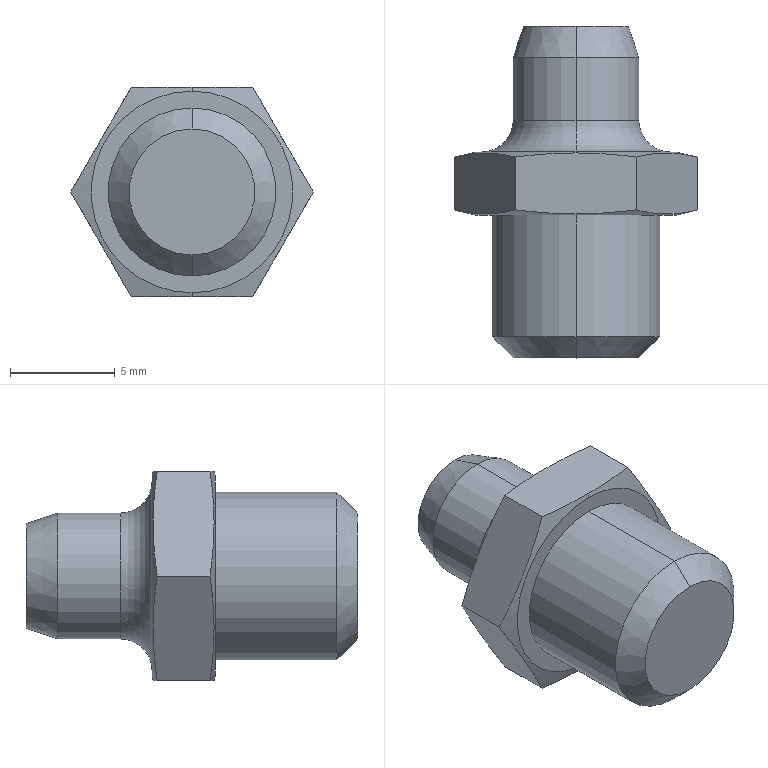Part | SolidWorks | features RevCut 2, Chamfer 1, Extrusion 1, ICE 1, Revolution 1 | 1 solid | 29 faces | box 11.547 x 15.8 x 10 mm | volume 760.457 mm3 | plane 11 | cone 10 | cylinder 4 | sphere 2 | torus 2 | commonest cylinder face diameters 6 x2 8 x2
STEP:
#1=CARTESIAN_POINT('',(0.,15.8,-0.8829));
#2=VERTEX_POINT('',#1);
#3=CARTESIAN_POINT('',(0.,15.8,0.8829));
#4=VERTEX_POINT('',#3);
#5=CARTESIAN_POINT('',(0.,15.8,0.));
#6=DIRECTION('',(0.,1.,0.));
#7=DIRECTION('',(0.,0.,1.));
#8=AXIS2_PLACEMENT_3D('',#5,#6,#7);
#9=CIRCLE('',#8,0.8829);
#10=EDGE_CURVE('',#2,#4,#9,.T.);
#11=ORIENTED_EDGE('',*,*,#10,.T.);
#12=CARTESIAN_POINT('',(0.,15.018,1.293));
#13=VERTEX_POINT('',#12);
#14=CARTESIAN_POINT('',(0.,15.018,1.293));
#15=DIRECTION('',(0.,-0.8855,0.4646));
#16=VECTOR('',#15,1000.);
#17=LINE('',#14,#16);
#18=EDGE_CURVE('',#4,#13,#17,.T.);
#19=ORIENTED_EDGE('',*,*,#18,.T.);
#20=CARTESIAN_POINT('',(0.,15.018,-1.293));
#21=VERTEX_POINT('',#20);
#22=CARTESIAN_POINT('',(0.,15.018,0.));
#23=DIRECTION('',(0.,1.,0.));
#24=DIRECTION('',(0.,0.,1.));
#25=AXIS2_PLACEMENT_3D('',#22,#23,#24);
#26=CIRCLE('',#25,1.293);
#27=EDGE_CURVE('',#21,#13,#26,.T.);
#28=ORIENTED_EDGE('',*,*,#27,.F.);
#29=CARTESIAN_POINT('',(0.,15.018,-1.293));
#30=DIRECTION('',(0.,-0.8855,-0.4646));
#31=VECTOR('',#30,1000.);
#32=LINE('',#29,#31);
#33=EDGE_CURVE('',#2,#21,#32,.T.);
#34=ORIENTED_EDGE('',*,*,#33,.F.);
#35=EDGE_LOOP('',(#11,#19,#28,#34));
#36=FACE_OUTER_BOUND('',#35,.T.);
#37=CARTESIAN_POINT('',(0.,15.018,0.));
#38=DIRECTION('',(0.,-1.,0.));
#39=DIRECTION('',(0.,0.,-1.));
#40=AXIS2_PLACEMENT_3D('',#37,#38,#39);
#41=CONICAL_SURFACE('',#40,1.293,0.4832);
#42=ADVANCED_FACE('',(#36),#41,.F.);
#43=CARTESIAN_POINT('',(0.,15.018,0.));
#44=DIRECTION('',(0.,1.,0.));
#45=DIRECTION('',(0.,0.,1.));
#46=AXIS2_PLACEMENT_3D('',#43,#44,#45);
#47=CIRCLE('',#46,1.293);
#48=EDGE_CURVE('',#13,#21,#47,.T.);
#49=ORIENTED_EDGE('',*,*,#48,.T.);
#50=CARTESIAN_POINT('',(0.,15.8,-0.02012));
#51=VERTEX_POINT('',#50);
#52=CARTESIAN_POINT('',(0.,14.34,0.));
#53=DIRECTION('',(1.,0.,0.));
#54=DIRECTION('',(0.,0.,-1.));
#55=AXIS2_PLACEMENT_3D('',#52,#53,#54);
#56=CIRCLE('',#55,1.46);
#57=EDGE_CURVE('',#21,#51,#56,.T.);
#58=ORIENTED_EDGE('',*,*,#57,.T.);
#59=CARTESIAN_POINT('',(0.,15.8,0.02012));
#60=VERTEX_POINT('',#59);
#61=CARTESIAN_POINT('',(0.,15.8,0.));
#62=DIRECTION('',(0.,1.,0.));
#63=DIRECTION('',(0.,0.,1.));
#64=AXIS2_PLACEMENT_3D('',#61,#62,#63);
#65=CIRCLE('',#64,0.02012);
#66=EDGE_CURVE('',#60,#51,#65,.T.);
#67=ORIENTED_EDGE('',*,*,#66,.F.);
#68=CARTESIAN_POINT('',(0.,14.34,0.));
#69=DIRECTION('',(-1.,0.,0.));
#70=DIRECTION('',(0.,0.,1.));
#71=AXIS2_PLACEMENT_3D('',#68,#69,#70);
#72=CIRCLE('',#71,1.46);
#73=EDGE_CURVE('',#13,#60,#72,.T.);
#74=ORIENTED_EDGE('',*,*,#73,.F.);
#75=EDGE_LOOP('',(#49,#58,#67,#74));
#76=FACE_OUTER_BOUND('',#75,.T.);
#77=CARTESIAN_POINT('',(0.,14.34,0.));
#78=DIRECTION('',(1.,0.,0.));
#79=DIRECTION('',(0.,0.,1.));
#80=AXIS2_PLACEMENT_3D('',#77,#78,#79);
#81=SPHERICAL_SURFACE('',#80,1.46);
#82=ADVANCED_FACE('',(#76),#81,.T.);
#83=CARTESIAN_POINT('',(0.,0.,-3.));
#84=VERTEX_POINT('',#83);
#85=CARTESIAN_POINT('',(0.,0.,3.));
#86=VERTEX_POINT('',#85);
#87=CARTESIAN_POINT('',(0.,0.,0.));
#88=DIRECTION('',(0.,-1.,0.));
#89=DIRECTION('',(0.,0.,1.));
#90=AXIS2_PLACEMENT_3D('',#87,#88,#89);
#91=CIRCLE('',#90,3.);
#92=EDGE_CURVE('',#84,#86,#91,.T.);
#93=ORIENTED_EDGE('',*,*,#92,.F.);
#94=CARTESIAN_POINT('',(0.,1.,-4.));
#95=VERTEX_POINT('',#94);
#96=CARTESIAN_POINT('',(0.,1.,-4.));
#97=DIRECTION('',(0.,0.7071,-0.7071));
#98=VECTOR('',#97,1000.);
#99=LINE('',#96,#98);
#100=EDGE_CURVE('',#84,#95,#99,.T.);
#101=ORIENTED_EDGE('',*,*,#100,.T.);
#102=CARTESIAN_POINT('',(0.,1.,4.));
#103=VERTEX_POINT('',#102);
#104=CARTESIAN_POINT('',(0.,1.,0.));
#105=DIRECTION('',(0.,1.,0.));
#106=DIRECTION('',(0.,0.,1.));
#107=AXIS2_PLACEMENT_3D('',#104,#105,#106);
#108=CIRCLE('',#107,4.);
#109=EDGE_CURVE('',#103,#95,#108,.T.);
#110=ORIENTED_EDGE('',*,*,#109,.F.);
#111=CARTESIAN_POINT('',(0.,1.,4.));
#112=DIRECTION('',(0.,0.7071,0.7071));
#113=VECTOR('',#112,1000.);
#114=LINE('',#111,#113);
#115=EDGE_CURVE('',#86,#103,#114,.T.);
#116=ORIENTED_EDGE('',*,*,#115,.F.);
#117=EDGE_LOOP('',(#93,#101,#110,#116));
#118=FACE_OUTER_BOUND('',#117,.T.);
#119=CARTESIAN_POINT('',(0.,1.,0.));
#120=DIRECTION('',(0.,1.,0.));
#121=DIRECTION('',(0.,0.,1.));
#122=AXIS2_PLACEMENT_3D('',#119,#120,#121);
#123=CONICAL_SURFACE('',#122,4.,0.7854);
#124=ADVANCED_FACE('',(#118),#123,.T.);
#125=CARTESIAN_POINT('',(0.,6.8,4.));
#126=VERTEX_POINT('',#125);
#127=CARTESIAN_POINT('',(0.,6.8,-4.));
#128=VERTEX_POINT('',#127);
#129=CARTESIAN_POINT('',(0.,6.8,0.));
#130=DIRECTION('',(0.,1.,0.));
#131=DIRECTION('',(0.,0.,1.));
#132=AXIS2_PLACEMENT_3D('',#129,#130,#131);
#133=CIRCLE('',#132,4.);
#134=EDGE_CURVE('',#126,#128,#133,.T.);
#135=ORIENTED_EDGE('',*,*,#134,.F.);
#136=CARTESIAN_POINT('',(0.,6.8,4.));
#137=DIRECTION('',(0.,-1.,0.));
#138=VECTOR('',#137,1000.);
#139=LINE('',#136,#138);
#140=EDGE_CURVE('',#126,#103,#139,.T.);
#141=ORIENTED_EDGE('',*,*,#140,.T.);
#142=ORIENTED_EDGE('',*,*,#109,.T.);
#143=CARTESIAN_POINT('',(0.,6.8,-4.));
#144=DIRECTION('',(0.,-1.,0.));
#145=VECTOR('',#144,1000.);
#146=LINE('',#143,#145);
#147=EDGE_CURVE('',#128,#95,#146,.T.);
#148=ORIENTED_EDGE('',*,*,#147,.F.);
#149=EDGE_LOOP('',(#135,#141,#142,#148));
#150=FACE_OUTER_BOUND('',#149,.T.);
#151=CARTESIAN_POINT('',(0.,6.8,0.));
#152=DIRECTION('',(0.,-1.,0.));
#153=DIRECTION('',(0.,0.,-1.));
#154=AXIS2_PLACEMENT_3D('',#151,#152,#153);
#155=CYLINDRICAL_SURFACE('',#154,4.);
#156=ADVANCED_FACE('',(#150),#155,.T.);
#157=CARTESIAN_POINT('',(0.,6.8,4.8));
#158=VERTEX_POINT('',#157);
#159=CARTESIAN_POINT('',(0.,6.8,-4.8));
#160=VERTEX_POINT('',#159);
#161=CARTESIAN_POINT('',(0.,6.8,0.));
#162=DIRECTION('',(0.,1.,0.));
#163=DIRECTION('',(0.,0.,1.));
#164=AXIS2_PLACEMENT_3D('',#161,#162,#163);
#165=CIRCLE('',#164,4.8);
#166=EDGE_CURVE('',#158,#160,#165,.T.);
#167=ORIENTED_EDGE('',*,*,#166,.T.);
#168=CARTESIAN_POINT('',(0.,6.85,-5.));
#169=VERTEX_POINT('',#168);
#170=CARTESIAN_POINT('',(0.,7.3,-6.8));
#171=DIRECTION('',(0.,0.2425,-0.9701));
#172=VECTOR('',#171,1000.);
#173=LINE('',#170,#172);
#174=EDGE_CURVE('',#160,#169,#173,.T.);
#175=ORIENTED_EDGE('',*,*,#174,.T.);
#176=CARTESIAN_POINT('',(2.887,7.043,-5.));
#177=VERTEX_POINT('',#176);
#178=CARTESIAN_POINT('',(0.,6.85,-5.));
#179=CARTESIAN_POINT('',(0.9585,6.85,-5.));
#180=CARTESIAN_POINT('',(1.929,6.924,-5.));
#181=CARTESIAN_POINT('',(2.887,7.043,-5.));
#182=B_SPLINE_CURVE_WITH_KNOTS('',3,(#178,#179,#180,#181),.UNSPECIFIED.,.F.,.F.,(4,4),(0.008769,0.01162),.UNSPECIFIED.);
#183=EDGE_CURVE('',#169,#177,#182,.T.);
#184=ORIENTED_EDGE('',*,*,#183,.T.);
#185=CARTESIAN_POINT('',(5.774,7.043,0.));
#186=VERTEX_POINT('',#185);
#187=CARTESIAN_POINT('',(2.887,7.043,-5.));
#188=CARTESIAN_POINT('',(3.368,6.923,-4.167));
#189=CARTESIAN_POINT('',(4.33,6.777,-2.5));
#190=CARTESIAN_POINT('',(5.292,6.923,-0.8333));
#191=CARTESIAN_POINT('',(5.774,7.043,0.));
#192=B_SPLINE_CURVE_WITH_KNOTS('',3,(#187,#188,#189,#190,#191),.UNSPECIFIED.,.F.,.F.,(4,1,4),(0.000000231,0.002887,0.005774),.UNSPECIFIED.);
#193=EDGE_CURVE('',#177,#186,#192,.T.);
#194=ORIENTED_EDGE('',*,*,#193,.T.);
#195=CARTESIAN_POINT('',(2.887,7.043,5.));
#196=VERTEX_POINT('',#195);
#197=CARTESIAN_POINT('',(5.774,7.043,0.));
#198=CARTESIAN_POINT('',(5.292,6.923,0.8333));
#199=CARTESIAN_POINT('',(4.33,6.777,2.5));
#200=CARTESIAN_POINT('',(3.368,6.923,4.167));
#201=CARTESIAN_POINT('',(2.887,7.043,5.));
#202=B_SPLINE_CURVE_WITH_KNOTS('',3,(#197,#198,#199,#200,#201),.UNSPECIFIED.,.F.,.F.,(4,1,4),(0.000000231,0.002887,0.005774),.UNSPECIFIED.);
#203=EDGE_CURVE('',#186,#196,#202,.T.);
#204=ORIENTED_EDGE('',*,*,#203,.T.);
#205=CARTESIAN_POINT('',(0.,6.85,5.));
#206=VERTEX_POINT('',#205);
#207=CARTESIAN_POINT('',(2.887,7.043,5.));
#208=CARTESIAN_POINT('',(1.931,6.924,5.));
#209=CARTESIAN_POINT('',(0.9699,6.85,5.));
#210=CARTESIAN_POINT('',(0.,6.85,5.));
#211=B_SPLINE_CURVE_WITH_KNOTS('',3,(#207,#208,#209,#210),.UNSPECIFIED.,.F.,.F.,(4,4),(0.00588,0.008769),.UNSPECIFIED.);
#212=EDGE_CURVE('',#196,#206,#211,.T.);
#213=ORIENTED_EDGE('',*,*,#212,.T.);
#214=CARTESIAN_POINT('',(0.,7.3,6.8));
#215=DIRECTION('',(0.,0.2425,0.9701));
#216=VECTOR('',#215,1000.);
#217=LINE('',#214,#216);
#218=EDGE_CURVE('',#158,#206,#217,.T.);
#219=ORIENTED_EDGE('',*,*,#218,.F.);
#220=EDGE_LOOP('',(#167,#175,#184,#194,#204,#213,#219));
#221=FACE_OUTER_BOUND('',#220,.T.);
#222=CARTESIAN_POINT('',(0.,7.3,0.));
#223=DIRECTION('',(0.,1.,0.));
#224=DIRECTION('',(0.,0.,1.));
#225=AXIS2_PLACEMENT_3D('',#222,#223,#224);
#226=CONICAL_SURFACE('',#225,6.8,1.326);
#227=ADVANCED_FACE('',(#221),#226,.T.);
#228=CARTESIAN_POINT('',(0.,9.8,4.8));
#229=VERTEX_POINT('',#228);
#230=CARTESIAN_POINT('',(0.,9.8,-4.8));
#231=VERTEX_POINT('',#230);
#232=CARTESIAN_POINT('',(0.,9.8,0.));
#233=DIRECTION('',(0.,1.,0.));
#234=DIRECTION('',(0.,0.,1.));
#235=AXIS2_PLACEMENT_3D('',#232,#233,#234);
#236=CIRCLE('',#235,4.8);
#237=EDGE_CURVE('',#229,#231,#236,.T.);
#238=ORIENTED_EDGE('',*,*,#237,.F.);
#239=CARTESIAN_POINT('',(0.,9.75,5.));
#240=VERTEX_POINT('',#239);
#241=CARTESIAN_POINT('',(0.,9.8,4.8));
#242=DIRECTION('',(0.,-0.2425,0.9701));
#243=VECTOR('',#242,1000.);
#244=LINE('',#241,#243);
#245=EDGE_CURVE('',#229,#240,#244,.T.);
#246=ORIENTED_EDGE('',*,*,#245,.T.);
#247=CARTESIAN_POINT('',(2.887,9.557,5.));
#248=VERTEX_POINT('',#247);
#249=CARTESIAN_POINT('',(0.,9.75,5.));
#250=CARTESIAN_POINT('',(0.9585,9.75,5.));
#251=CARTESIAN_POINT('',(1.929,9.676,5.));
#252=CARTESIAN_POINT('',(2.887,9.557,5.));
#253=B_SPLINE_CURVE_WITH_KNOTS('',3,(#249,#250,#251,#252),.UNSPECIFIED.,.F.,.F.,(4,4),(0.008769,0.01162),.UNSPECIFIED.);
#254=EDGE_CURVE('',#240,#248,#253,.T.);
#255=ORIENTED_EDGE('',*,*,#254,.T.);
#256=CARTESIAN_POINT('',(5.774,9.557,0.));
#257=VERTEX_POINT('',#256);
#258=CARTESIAN_POINT('',(2.887,9.557,5.));
#259=CARTESIAN_POINT('',(3.368,9.677,4.167));
#260=CARTESIAN_POINT('',(4.33,9.823,2.5));
#261=CARTESIAN_POINT('',(5.292,9.677,0.8333));
#262=CARTESIAN_POINT('',(5.774,9.557,0.));
#263=B_SPLINE_CURVE_WITH_KNOTS('',3,(#258,#259,#260,#261,#262),.UNSPECIFIED.,.F.,.F.,(4,1,4),(0.000000231,0.002887,0.005774),.UNSPECIFIED.);
#264=EDGE_CURVE('',#248,#257,#263,.T.);
#265=ORIENTED_EDGE('',*,*,#264,.T.);
#266=CARTESIAN_POINT('',(2.887,9.557,-5.));
#267=VERTEX_POINT('',#266);
#268=CARTESIAN_POINT('',(5.774,9.557,0.));
#269=CARTESIAN_POINT('',(5.292,9.677,-0.8333));
#270=CARTESIAN_POINT('',(4.33,9.823,-2.5));
#271=CARTESIAN_POINT('',(3.368,9.677,-4.167));
#272=CARTESIAN_POINT('',(2.887,9.557,-5.));
#273=B_SPLINE_CURVE_WITH_KNOTS('',3,(#268,#269,#270,#271,#272),.UNSPECIFIED.,.F.,.F.,(4,1,4),(0.000000231,0.002887,0.005774),.UNSPECIFIED.);
#274=EDGE_CURVE('',#257,#267,#273,.T.);
#275=ORIENTED_EDGE('',*,*,#274,.T.);
#276=CARTESIAN_POINT('',(0.,9.75,-5.));
#277=VERTEX_POINT('',#276);
#278=CARTESIAN_POINT('',(2.887,9.557,-5.));
#279=CARTESIAN_POINT('',(1.931,9.676,-5.));
#280=CARTESIAN_POINT('',(0.9699,9.75,-5.));
#281=CARTESIAN_POINT('',(0.,9.75,-5.));
#282=B_SPLINE_CURVE_WITH_KNOTS('',3,(#278,#279,#280,#281),.UNSPECIFIED.,.F.,.F.,(4,4),(0.00588,0.008769),.UNSPECIFIED.);
#283=EDGE_CURVE('',#267,#277,#282,.T.);
#284=ORIENTED_EDGE('',*,*,#283,.T.);
#285=CARTESIAN_POINT('',(0.,9.8,-4.8));
#286=DIRECTION('',(0.,-0.2425,-0.9701));
#287=VECTOR('',#286,1000.);
#288=LINE('',#285,#287);
#289=EDGE_CURVE('',#231,#277,#288,.T.);
#290=ORIENTED_EDGE('',*,*,#289,.F.);
#291=EDGE_LOOP('',(#238,#246,#255,#265,#275,#284,#290));
#292=FACE_OUTER_BOUND('',#291,.T.);
#293=CARTESIAN_POINT('',(0.,9.8,0.));
#294=DIRECTION('',(0.,-1.,0.));
#295=DIRECTION('',(0.,0.,-1.));
#296=AXIS2_PLACEMENT_3D('',#293,#294,#295);
#297=CONICAL_SURFACE('',#296,4.8,1.326);
#298=ADVANCED_FACE('',(#292),#297,.T.);
#299=CARTESIAN_POINT('',(0.,15.8,-2.5));
#300=VERTEX_POINT('',#299);
#301=CARTESIAN_POINT('',(0.,15.8,2.5));
#302=VERTEX_POINT('',#301);
#303=CARTESIAN_POINT('',(0.,15.8,0.));
#304=DIRECTION('',(0.,-1.,0.));
#305=DIRECTION('',(0.,0.,-1.));
#306=AXIS2_PLACEMENT_3D('',#303,#304,#305);
#307=CIRCLE('',#306,2.5);
#308=EDGE_CURVE('',#300,#302,#307,.T.);
#309=ORIENTED_EDGE('',*,*,#308,.T.);
#310=CARTESIAN_POINT('',(0.,14.3,3.));
#311=VERTEX_POINT('',#310);
#312=CARTESIAN_POINT('',(0.,15.8,2.5));
#313=DIRECTION('',(0.,-0.9487,0.3162));
#314=VECTOR('',#313,1000.);
#315=LINE('',#312,#314);
#316=EDGE_CURVE('',#302,#311,#315,.T.);
#317=ORIENTED_EDGE('',*,*,#316,.T.);
#318=CARTESIAN_POINT('',(0.,14.3,-3.));
#319=VERTEX_POINT('',#318);
#320=CARTESIAN_POINT('',(0.,14.3,0.));
#321=DIRECTION('',(0.,-1.,0.));
#322=DIRECTION('',(0.,0.,-1.));
#323=AXIS2_PLACEMENT_3D('',#320,#321,#322);
#324=CIRCLE('',#323,3.);
#325=EDGE_CURVE('',#319,#311,#324,.T.);
#326=ORIENTED_EDGE('',*,*,#325,.F.);
#327=CARTESIAN_POINT('',(0.,15.8,-2.5));
#328=DIRECTION('',(0.,-0.9487,-0.3162));
#329=VECTOR('',#328,1000.);
#330=LINE('',#327,#329);
#331=EDGE_CURVE('',#300,#319,#330,.T.);
#332=ORIENTED_EDGE('',*,*,#331,.F.);
#333=EDGE_LOOP('',(#309,#317,#326,#332));
#334=FACE_OUTER_BOUND('',#333,.T.);
#335=CARTESIAN_POINT('',(0.,15.8,0.));
#336=DIRECTION('',(0.,-1.,0.));
#337=DIRECTION('',(0.,0.,-1.));
#338=AXIS2_PLACEMENT_3D('',#335,#336,#337);
#339=CONICAL_SURFACE('',#338,2.5,0.3218);
#340=ADVANCED_FACE('',(#334),#339,.T.);
#341=ORIENTED_EDGE('',*,*,#325,.T.);
#342=CARTESIAN_POINT('',(0.,11.3,3.));
#343=VERTEX_POINT('',#342);
#344=CARTESIAN_POINT('',(0.,-1.88,3.));
#345=DIRECTION('',(0.,-1.,0.));
#346=VECTOR('',#345,1000.);
#347=LINE('',#344,#346);
#348=EDGE_CURVE('',#311,#343,#347,.T.);
#349=ORIENTED_EDGE('',*,*,#348,.T.);
#350=CARTESIAN_POINT('',(0.,11.3,-3.));
#351=VERTEX_POINT('',#350);
#352=CARTESIAN_POINT('',(0.,11.3,0.));
#353=DIRECTION('',(0.,-1.,0.));
#354=DIRECTION('',(0.,0.,-1.));
#355=AXIS2_PLACEMENT_3D('',#352,#353,#354);
#356=CIRCLE('',#355,3.);
#357=EDGE_CURVE('',#351,#343,#356,.T.);
#358=ORIENTED_EDGE('',*,*,#357,.F.);
#359=CARTESIAN_POINT('',(0.,-1.88,-3.));
#360=DIRECTION('',(0.,-1.,0.));
#361=VECTOR('',#360,1000.);
#362=LINE('',#359,#361);
#363=EDGE_CURVE('',#319,#351,#362,.T.);
#364=ORIENTED_EDGE('',*,*,#363,.F.);
#365=EDGE_LOOP('',(#341,#349,#358,#364));
#366=FACE_OUTER_BOUND('',#365,.T.);
#367=CARTESIAN_POINT('',(0.,-1.88,0.));
#368=DIRECTION('',(0.,-1.,0.));
#369=DIRECTION('',(0.,0.,-1.));
#370=AXIS2_PLACEMENT_3D('',#367,#368,#369);
#371=CYLINDRICAL_SURFACE('',#370,3.);
#372=ADVANCED_FACE('',(#366),#371,.T.);
#373=CARTESIAN_POINT('',(0.,9.8,4.5));
#374=VERTEX_POINT('',#373);
#375=CARTESIAN_POINT('',(0.,9.8,-4.5));
#376=VERTEX_POINT('',#375);
#377=CARTESIAN_POINT('',(0.,9.8,0.));
#378=DIRECTION('',(0.,-1.,0.));
#379=DIRECTION('',(0.,0.,-1.));
#380=AXIS2_PLACEMENT_3D('',#377,#378,#379);
#381=CIRCLE('',#380,4.5);
#382=EDGE_CURVE('',#374,#376,#381,.T.);
#383=ORIENTED_EDGE('',*,*,#382,.F.);
#384=CARTESIAN_POINT('',(0.,11.3,4.5));
#385=DIRECTION('',(1.,0.,0.));
#386=DIRECTION('',(0.,0.,-1.));
#387=AXIS2_PLACEMENT_3D('',#384,#385,#386);
#388=CIRCLE('',#387,1.5);
#389=EDGE_CURVE('',#374,#343,#388,.T.);
#390=ORIENTED_EDGE('',*,*,#389,.T.);
#391=CARTESIAN_POINT('',(0.,11.3,0.));
#392=DIRECTION('',(0.,-1.,0.));
#393=DIRECTION('',(0.,0.,-1.));
#394=AXIS2_PLACEMENT_3D('',#391,#392,#393);
#395=CIRCLE('',#394,3.);
#396=EDGE_CURVE('',#343,#351,#395,.T.);
#397=ORIENTED_EDGE('',*,*,#396,.T.);
#398=CARTESIAN_POINT('',(0.,11.3,-4.5));
#399=DIRECTION('',(-1.,0.,0.));
#400=DIRECTION('',(0.,0.,1.));
#401=AXIS2_PLACEMENT_3D('',#398,#399,#400);
#402=CIRCLE('',#401,1.5);
#403=EDGE_CURVE('',#376,#351,#402,.T.);
#404=ORIENTED_EDGE('',*,*,#403,.F.);
#405=EDGE_LOOP('',(#383,#390,#397,#404));
#406=FACE_OUTER_BOUND('',#405,.T.);
#407=CARTESIAN_POINT('',(0.,11.3,0.));
#408=DIRECTION('',(0.,-1.,0.));
#409=DIRECTION('',(0.,0.,-1.));
#410=AXIS2_PLACEMENT_3D('',#407,#408,#409);
#411=TOROIDAL_SURFACE('',#410,4.5,1.5);
#412=ADVANCED_FACE('',(#406),#411,.F.);
#413=CARTESIAN_POINT('',(0.,9.8,0.));
#414=DIRECTION('',(0.,-1.,0.));
#415=DIRECTION('',(0.,0.,-1.));
#416=AXIS2_PLACEMENT_3D('',#413,#414,#415);
#417=CIRCLE('',#416,4.5);
#418=EDGE_CURVE('',#376,#374,#417,.T.);
#419=ORIENTED_EDGE('',*,*,#418,.T.);
#420=ORIENTED_EDGE('',*,*,#382,.T.);
#421=EDGE_LOOP('',(#419,#420));
#422=FACE_BOUND('',#421,.T.);
#423=CARTESIAN_POINT('',(0.,9.8,0.));
#424=DIRECTION('',(0.,1.,0.));
#425=DIRECTION('',(0.,0.,1.));
#426=AXIS2_PLACEMENT_3D('',#423,#424,#425);
#427=CIRCLE('',#426,4.8);
#428=EDGE_CURVE('',#231,#229,#427,.T.);
#429=ORIENTED_EDGE('',*,*,#428,.T.);
#430=ORIENTED_EDGE('',*,*,#237,.T.);
#431=EDGE_LOOP('',(#429,#430));
#432=FACE_OUTER_BOUND('',#431,.T.);
#433=CARTESIAN_POINT('',(0.,9.8,0.));
#434=DIRECTION('',(0.,1.,0.));
#435=DIRECTION('',(0.,0.,1.));
#436=AXIS2_PLACEMENT_3D('',#433,#434,#435);
#437=PLANE('',#436);
#438=ADVANCED_FACE('',(#422,#432),#437,.T.);
#439=ORIENTED_EDGE('',*,*,#389,.F.);
#440=ORIENTED_EDGE('',*,*,#418,.F.);
#441=ORIENTED_EDGE('',*,*,#403,.T.);
#442=ORIENTED_EDGE('',*,*,#357,.T.);
#443=EDGE_LOOP('',(#439,#440,#441,#442));
#444=FACE_OUTER_BOUND('',#443,.T.);
#445=CARTESIAN_POINT('',(0.,11.3,0.));
#446=DIRECTION('',(0.,-1.,0.));
#447=DIRECTION('',(0.,0.,-1.));
#448=AXIS2_PLACEMENT_3D('',#445,#446,#447);
#449=TOROIDAL_SURFACE('',#448,4.5,1.5);
#450=ADVANCED_FACE('',(#444),#449,.F.);
#451=ORIENTED_EDGE('',*,*,#348,.F.);
#452=CARTESIAN_POINT('',(0.,14.3,0.));
#453=DIRECTION('',(0.,-1.,0.));
#454=DIRECTION('',(0.,0.,-1.));
#455=AXIS2_PLACEMENT_3D('',#452,#453,#454);
#456=CIRCLE('',#455,3.);
#457=EDGE_CURVE('',#311,#319,#456,.T.);
#458=ORIENTED_EDGE('',*,*,#457,.T.);
#459=ORIENTED_EDGE('',*,*,#363,.T.);
#460=ORIENTED_EDGE('',*,*,#396,.F.);
#461=EDGE_LOOP('',(#451,#458,#459,#460));
#462=FACE_OUTER_BOUND('',#461,.T.);
#463=CARTESIAN_POINT('',(0.,-1.88,0.));
#464=DIRECTION('',(0.,-1.,0.));
#465=DIRECTION('',(0.,0.,-1.));
#466=AXIS2_PLACEMENT_3D('',#463,#464,#465);
#467=CYLINDRICAL_SURFACE('',#466,3.);
#468=ADVANCED_FACE('',(#462),#467,.T.);
#469=ORIENTED_EDGE('',*,*,#316,.F.);
#470=CARTESIAN_POINT('',(0.,15.8,0.));
#471=DIRECTION('',(0.,-1.,0.));
#472=DIRECTION('',(0.,0.,-1.));
#473=AXIS2_PLACEMENT_3D('',#470,#471,#472);
#474=CIRCLE('',#473,2.5);
#475=EDGE_CURVE('',#302,#300,#474,.T.);
#476=ORIENTED_EDGE('',*,*,#475,.T.);
#477=ORIENTED_EDGE('',*,*,#331,.T.);
#478=ORIENTED_EDGE('',*,*,#457,.F.);
#479=EDGE_LOOP('',(#469,#476,#477,#478));
#480=FACE_OUTER_BOUND('',#479,.T.);
#481=CARTESIAN_POINT('',(0.,15.8,0.));
#482=DIRECTION('',(0.,-1.,0.));
#483=DIRECTION('',(0.,0.,-1.));
#484=AXIS2_PLACEMENT_3D('',#481,#482,#483);
#485=CONICAL_SURFACE('',#484,2.5,0.3218);
#486=ADVANCED_FACE('',(#480),#485,.T.);
#487=ORIENTED_EDGE('',*,*,#10,.F.);
#488=CARTESIAN_POINT('',(0.,15.8,0.));
#489=DIRECTION('',(0.,1.,0.));
#490=DIRECTION('',(0.,0.,1.));
#491=AXIS2_PLACEMENT_3D('',#488,#489,#490);
#492=CIRCLE('',#491,0.8829);
#493=EDGE_CURVE('',#4,#2,#492,.T.);
#494=ORIENTED_EDGE('',*,*,#493,.F.);
#495=EDGE_LOOP('',(#487,#494));
#496=FACE_BOUND('',#495,.T.);
#497=ORIENTED_EDGE('',*,*,#308,.F.);
#498=ORIENTED_EDGE('',*,*,#475,.F.);
#499=EDGE_LOOP('',(#497,#498));
#500=FACE_OUTER_BOUND('',#499,.T.);
#501=CARTESIAN_POINT('',(0.,15.8,0.));
#502=DIRECTION('',(0.,-1.,0.));
#503=DIRECTION('',(0.,0.,-1.));
#504=AXIS2_PLACEMENT_3D('',#501,#502,#503);
#505=PLANE('',#504);
#506=ADVANCED_FACE('',(#496,#500),#505,.F.);
#507=ORIENTED_EDGE('',*,*,#245,.F.);
#508=ORIENTED_EDGE('',*,*,#428,.F.);
#509=ORIENTED_EDGE('',*,*,#289,.T.);
#510=CARTESIAN_POINT('',(-2.887,9.557,-5.));
#511=VERTEX_POINT('',#510);
#512=CARTESIAN_POINT('',(0.,9.75,-5.));
#513=CARTESIAN_POINT('',(-0.9585,9.75,-5.));
#514=CARTESIAN_POINT('',(-1.929,9.676,-5.));
#515=CARTESIAN_POINT('',(-2.887,9.557,-5.));
#516=B_SPLINE_CURVE_WITH_KNOTS('',3,(#512,#513,#514,#515),.UNSPECIFIED.,.F.,.F.,(4,4),(0.008769,0.01162),.UNSPECIFIED.);
#517=EDGE_CURVE('',#277,#511,#516,.T.);
#518=ORIENTED_EDGE('',*,*,#517,.T.);
#519=CARTESIAN_POINT('',(-5.774,9.557,0.));
#520=VERTEX_POINT('',#519);
#521=CARTESIAN_POINT('',(-2.887,9.557,-5.));
#522=CARTESIAN_POINT('',(-3.368,9.677,-4.167));
#523=CARTESIAN_POINT('',(-4.33,9.823,-2.5));
#524=CARTESIAN_POINT('',(-5.292,9.677,-0.8333));
#525=CARTESIAN_POINT('',(-5.774,9.557,0.));
#526=B_SPLINE_CURVE_WITH_KNOTS('',3,(#521,#522,#523,#524,#525),.UNSPECIFIED.,.F.,.F.,(4,1,4),(0.000000231,0.002887,0.005774),.UNSPECIFIED.);
#527=EDGE_CURVE('',#511,#520,#526,.T.);
#528=ORIENTED_EDGE('',*,*,#527,.T.);
#529=CARTESIAN_POINT('',(-2.887,9.557,5.));
#530=VERTEX_POINT('',#529);
#531=CARTESIAN_POINT('',(-5.774,9.557,0.));
#532=CARTESIAN_POINT('',(-5.292,9.677,0.8333));
#533=CARTESIAN_POINT('',(-4.33,9.823,2.5));
#534=CARTESIAN_POINT('',(-3.368,9.677,4.167));
#535=CARTESIAN_POINT('',(-2.887,9.557,5.));
#536=B_SPLINE_CURVE_WITH_KNOTS('',3,(#531,#532,#533,#534,#535),.UNSPECIFIED.,.F.,.F.,(4,1,4),(0.000000231,0.002887,0.005774),.UNSPECIFIED.);
#537=EDGE_CURVE('',#520,#530,#536,.T.);
#538=ORIENTED_EDGE('',*,*,#537,.T.);
#539=CARTESIAN_POINT('',(-2.887,9.557,5.));
#540=CARTESIAN_POINT('',(-1.931,9.676,5.));
#541=CARTESIAN_POINT('',(-0.9699,9.75,5.));
#542=CARTESIAN_POINT('',(0.,9.75,5.));
#543=B_SPLINE_CURVE_WITH_KNOTS('',3,(#539,#540,#541,#542),.UNSPECIFIED.,.F.,.F.,(4,4),(0.00588,0.008769),.UNSPECIFIED.);
#544=EDGE_CURVE('',#530,#240,#543,.T.);
#545=ORIENTED_EDGE('',*,*,#544,.T.);
#546=EDGE_LOOP('',(#507,#508,#509,#518,#528,#538,#545));
#547=FACE_OUTER_BOUND('',#546,.T.);
#548=CARTESIAN_POINT('',(0.,9.8,0.));
#549=DIRECTION('',(0.,-1.,0.));
#550=DIRECTION('',(0.,0.,-1.));
#551=AXIS2_PLACEMENT_3D('',#548,#549,#550);
#552=CONICAL_SURFACE('',#551,4.8,1.326);
#553=ADVANCED_FACE('',(#547),#552,.T.);
#554=ORIENTED_EDGE('',*,*,#537,.F.);
#555=CARTESIAN_POINT('',(-5.774,7.043,0.));
#556=VERTEX_POINT('',#555);
#557=CARTESIAN_POINT('',(-5.774,9.8,0.));
#558=DIRECTION('',(0.,-1.,0.));
#559=VECTOR('',#558,1000.);
#560=LINE('',#557,#559);
#561=EDGE_CURVE('',#520,#556,#560,.T.);
#562=ORIENTED_EDGE('',*,*,#561,.T.);
#563=CARTESIAN_POINT('',(-2.887,7.043,5.));
#564=VERTEX_POINT('',#563);
#565=CARTESIAN_POINT('',(-2.887,7.043,5.));
#566=CARTESIAN_POINT('',(-3.368,6.923,4.167));
#567=CARTESIAN_POINT('',(-4.33,6.777,2.5));
#568=CARTESIAN_POINT('',(-5.292,6.923,0.8333));
#569=CARTESIAN_POINT('',(-5.774,7.043,0.));
#570=B_SPLINE_CURVE_WITH_KNOTS('',3,(#565,#566,#567,#568,#569),.UNSPECIFIED.,.F.,.F.,(4,1,4),(0.000000231,0.002887,0.005774),.UNSPECIFIED.);
#571=EDGE_CURVE('',#564,#556,#570,.T.);
#572=ORIENTED_EDGE('',*,*,#571,.F.);
#573=CARTESIAN_POINT('',(-2.887,9.8,5.));
#574=DIRECTION('',(0.,-1.,0.));
#575=VECTOR('',#574,1000.);
#576=LINE('',#573,#575);
#577=EDGE_CURVE('',#530,#564,#576,.T.);
#578=ORIENTED_EDGE('',*,*,#577,.F.);
#579=EDGE_LOOP('',(#554,#562,#572,#578));
#580=FACE_OUTER_BOUND('',#579,.T.);
#581=CARTESIAN_POINT('',(-5.774,9.8,0.));
#582=DIRECTION('',(0.866,0.,-0.5));
#583=DIRECTION('',(-0.5,0.,-0.866));
#584=AXIS2_PLACEMENT_3D('',#581,#582,#583);
#585=PLANE('',#584);
#586=ADVANCED_FACE('',(#580),#585,.F.);
#587=ORIENTED_EDGE('',*,*,#527,.F.);
#588=CARTESIAN_POINT('',(-2.887,7.043,-5.));
#589=VERTEX_POINT('',#588);
#590=CARTESIAN_POINT('',(-2.887,9.8,-5.));
#591=DIRECTION('',(0.,-1.,0.));
#592=VECTOR('',#591,1000.);
#593=LINE('',#590,#592);
#594=EDGE_CURVE('',#511,#589,#593,.T.);
#595=ORIENTED_EDGE('',*,*,#594,.T.);
#596=CARTESIAN_POINT('',(-5.774,7.043,0.));
#597=CARTESIAN_POINT('',(-5.292,6.923,-0.8333));
#598=CARTESIAN_POINT('',(-4.33,6.777,-2.5));
#599=CARTESIAN_POINT('',(-3.368,6.923,-4.167));
#600=CARTESIAN_POINT('',(-2.887,7.043,-5.));
#601=B_SPLINE_CURVE_WITH_KNOTS('',3,(#596,#597,#598,#599,#600),.UNSPECIFIED.,.F.,.F.,(4,1,4),(0.000000231,0.002887,0.005774),.UNSPECIFIED.);
#602=EDGE_CURVE('',#556,#589,#601,.T.);
#603=ORIENTED_EDGE('',*,*,#602,.F.);
#604=ORIENTED_EDGE('',*,*,#561,.F.);
#605=EDGE_LOOP('',(#587,#595,#603,#604));
#606=FACE_OUTER_BOUND('',#605,.T.);
#607=CARTESIAN_POINT('',(-2.887,9.8,-5.));
#608=DIRECTION('',(0.866,0.,0.5));
#609=DIRECTION('',(0.5,0.,-0.866));
#610=AXIS2_PLACEMENT_3D('',#607,#608,#609);
#611=PLANE('',#610);
#612=ADVANCED_FACE('',(#606),#611,.F.);
#613=ORIENTED_EDGE('',*,*,#283,.F.);
#614=CARTESIAN_POINT('',(2.887,9.8,-5.));
#615=DIRECTION('',(0.,-1.,0.));
#616=VECTOR('',#615,1000.);
#617=LINE('',#614,#616);
#618=EDGE_CURVE('',#267,#177,#617,.T.);
#619=ORIENTED_EDGE('',*,*,#618,.T.);
#620=ORIENTED_EDGE('',*,*,#183,.F.);
#621=CARTESIAN_POINT('',(-2.887,7.043,-5.));
#622=CARTESIAN_POINT('',(-1.931,6.924,-5.));
#623=CARTESIAN_POINT('',(-0.9699,6.85,-5.));
#624=CARTESIAN_POINT('',(0.,6.85,-5.));
#625=B_SPLINE_CURVE_WITH_KNOTS('',3,(#621,#622,#623,#624),.UNSPECIFIED.,.F.,.F.,(4,4),(0.00588,0.008769),.UNSPECIFIED.);
#626=EDGE_CURVE('',#589,#169,#625,.T.);
#627=ORIENTED_EDGE('',*,*,#626,.F.);
#628=ORIENTED_EDGE('',*,*,#594,.F.);
#629=ORIENTED_EDGE('',*,*,#517,.F.);
#630=EDGE_LOOP('',(#613,#619,#620,#627,#628,#629));
#631=FACE_OUTER_BOUND('',#630,.T.);
#632=CARTESIAN_POINT('',(2.887,9.8,-5.));
#633=DIRECTION('',(0.,0.,1.));
#634=DIRECTION('',(1.,0.,0.));
#635=AXIS2_PLACEMENT_3D('',#632,#633,#634);
#636=PLANE('',#635);
#637=ADVANCED_FACE('',(#631),#636,.F.);
#638=ORIENTED_EDGE('',*,*,#274,.F.);
#639=CARTESIAN_POINT('',(5.774,9.8,0.));
#640=DIRECTION('',(0.,-1.,0.));
#641=VECTOR('',#640,1000.);
#642=LINE('',#639,#641);
#643=EDGE_CURVE('',#257,#186,#642,.T.);
#644=ORIENTED_EDGE('',*,*,#643,.T.);
#645=ORIENTED_EDGE('',*,*,#193,.F.);
#646=ORIENTED_EDGE('',*,*,#618,.F.);
#647=EDGE_LOOP('',(#638,#644,#645,#646));
#648=FACE_OUTER_BOUND('',#647,.T.);
#649=CARTESIAN_POINT('',(5.774,9.8,0.));
#650=DIRECTION('',(-0.866,0.,0.5));
#651=DIRECTION('',(0.5,0.,0.866));
#652=AXIS2_PLACEMENT_3D('',#649,#650,#651);
#653=PLANE('',#652);
#654=ADVANCED_FACE('',(#648),#653,.F.);
#655=ORIENTED_EDGE('',*,*,#264,.F.);
#656=CARTESIAN_POINT('',(2.887,9.8,5.));
#657=DIRECTION('',(0.,-1.,0.));
#658=VECTOR('',#657,1000.);
#659=LINE('',#656,#658);
#660=EDGE_CURVE('',#248,#196,#659,.T.);
#661=ORIENTED_EDGE('',*,*,#660,.T.);
#662=ORIENTED_EDGE('',*,*,#203,.F.);
#663=ORIENTED_EDGE('',*,*,#643,.F.);
#664=EDGE_LOOP('',(#655,#661,#662,#663));
#665=FACE_OUTER_BOUND('',#664,.T.);
#666=CARTESIAN_POINT('',(2.887,9.8,5.));
#667=DIRECTION('',(-0.866,0.,-0.5));
#668=DIRECTION('',(-0.5,0.,0.866));
#669=AXIS2_PLACEMENT_3D('',#666,#667,#668);
#670=PLANE('',#669);
#671=ADVANCED_FACE('',(#665),#670,.F.);
#672=ORIENTED_EDGE('',*,*,#544,.F.);
#673=ORIENTED_EDGE('',*,*,#577,.T.);
#674=CARTESIAN_POINT('',(0.,6.85,5.));
#675=CARTESIAN_POINT('',(-0.9585,6.85,5.));
#676=CARTESIAN_POINT('',(-1.929,6.924,5.));
#677=CARTESIAN_POINT('',(-2.887,7.043,5.));
#678=B_SPLINE_CURVE_WITH_KNOTS('',3,(#674,#675,#676,#677),.UNSPECIFIED.,.F.,.F.,(4,4),(0.008769,0.01162),.UNSPECIFIED.);
#679=EDGE_CURVE('',#206,#564,#678,.T.);
#680=ORIENTED_EDGE('',*,*,#679,.F.);
#681=ORIENTED_EDGE('',*,*,#212,.F.);
#682=ORIENTED_EDGE('',*,*,#660,.F.);
#683=ORIENTED_EDGE('',*,*,#254,.F.);
#684=EDGE_LOOP('',(#672,#673,#680,#681,#682,#683));
#685=FACE_OUTER_BOUND('',#684,.T.);
#686=CARTESIAN_POINT('',(-2.887,9.8,5.));
#687=DIRECTION('',(0.,0.,-1.));
#688=DIRECTION('',(-1.,0.,0.));
#689=AXIS2_PLACEMENT_3D('',#686,#687,#688);
#690=PLANE('',#689);
#691=ADVANCED_FACE('',(#685),#690,.F.);
#692=ORIENTED_EDGE('',*,*,#174,.F.);
#693=CARTESIAN_POINT('',(0.,6.8,0.));
#694=DIRECTION('',(0.,1.,0.));
#695=DIRECTION('',(0.,0.,1.));
#696=AXIS2_PLACEMENT_3D('',#693,#694,#695);
#697=CIRCLE('',#696,4.8);
#698=EDGE_CURVE('',#160,#158,#697,.T.);
#699=ORIENTED_EDGE('',*,*,#698,.T.);
#700=ORIENTED_EDGE('',*,*,#218,.T.);
#701=ORIENTED_EDGE('',*,*,#679,.T.);
#702=ORIENTED_EDGE('',*,*,#571,.T.);
#703=ORIENTED_EDGE('',*,*,#602,.T.);
#704=ORIENTED_EDGE('',*,*,#626,.T.);
#705=EDGE_LOOP('',(#692,#699,#700,#701,#702,#703,#704));
#706=FACE_OUTER_BOUND('',#705,.T.);
#707=CARTESIAN_POINT('',(0.,7.3,0.));
#708=DIRECTION('',(0.,1.,0.));
#709=DIRECTION('',(0.,0.,1.));
#710=AXIS2_PLACEMENT_3D('',#707,#708,#709);
#711=CONICAL_SURFACE('',#710,6.8,1.326);
#712=ADVANCED_FACE('',(#706),#711,.T.);
#713=CARTESIAN_POINT('',(0.,0.,0.));
#714=DIRECTION('',(0.,-1.,0.));
#715=DIRECTION('',(0.,0.,1.));
#716=AXIS2_PLACEMENT_3D('',#713,#714,#715);
#717=CIRCLE('',#716,3.);
#718=EDGE_CURVE('',#86,#84,#717,.T.);
#719=ORIENTED_EDGE('',*,*,#718,.T.);
#720=ORIENTED_EDGE('',*,*,#92,.T.);
#721=EDGE_LOOP('',(#719,#720));
#722=FACE_OUTER_BOUND('',#721,.T.);
#723=CARTESIAN_POINT('',(0.,0.,0.));
#724=DIRECTION('',(0.,1.,0.));
#725=DIRECTION('',(0.,0.,1.));
#726=AXIS2_PLACEMENT_3D('',#723,#724,#725);
#727=PLANE('',#726);
#728=ADVANCED_FACE('',(#722),#727,.F.);
#729=ORIENTED_EDGE('',*,*,#140,.F.);
#730=CARTESIAN_POINT('',(0.,6.8,0.));
#731=DIRECTION('',(0.,1.,0.));
#732=DIRECTION('',(0.,0.,1.));
#733=AXIS2_PLACEMENT_3D('',#730,#731,#732);
#734=CIRCLE('',#733,4.);
#735=EDGE_CURVE('',#128,#126,#734,.T.);
#736=ORIENTED_EDGE('',*,*,#735,.F.);
#737=ORIENTED_EDGE('',*,*,#147,.T.);
#738=CARTESIAN_POINT('',(0.,1.,0.));
#739=DIRECTION('',(0.,1.,0.));
#740=DIRECTION('',(0.,0.,1.));
#741=AXIS2_PLACEMENT_3D('',#738,#739,#740);
#742=CIRCLE('',#741,4.);
#743=EDGE_CURVE('',#95,#103,#742,.T.);
#744=ORIENTED_EDGE('',*,*,#743,.T.);
#745=EDGE_LOOP('',(#729,#736,#737,#744));
#746=FACE_OUTER_BOUND('',#745,.T.);
#747=CARTESIAN_POINT('',(0.,6.8,0.));
#748=DIRECTION('',(0.,-1.,0.));
#749=DIRECTION('',(0.,0.,-1.));
#750=AXIS2_PLACEMENT_3D('',#747,#748,#749);
#751=CYLINDRICAL_SURFACE('',#750,4.);
#752=ADVANCED_FACE('',(#746),#751,.T.);
#753=ORIENTED_EDGE('',*,*,#735,.T.);
#754=ORIENTED_EDGE('',*,*,#134,.T.);
#755=EDGE_LOOP('',(#753,#754));
#756=FACE_BOUND('',#755,.T.);
#757=ORIENTED_EDGE('',*,*,#166,.F.);
#758=ORIENTED_EDGE('',*,*,#698,.F.);
#759=EDGE_LOOP('',(#757,#758));
#760=FACE_OUTER_BOUND('',#759,.T.);
#761=CARTESIAN_POINT('',(0.,6.8,0.));
#762=DIRECTION('',(0.,1.,0.));
#763=DIRECTION('',(0.,0.,1.));
#764=AXIS2_PLACEMENT_3D('',#761,#762,#763);
#765=PLANE('',#764);
#766=ADVANCED_FACE('',(#756,#760),#765,.F.);
#767=ORIENTED_EDGE('',*,*,#100,.F.);
#768=ORIENTED_EDGE('',*,*,#718,.F.);
#769=ORIENTED_EDGE('',*,*,#115,.T.);
#770=ORIENTED_EDGE('',*,*,#743,.F.);
#771=EDGE_LOOP('',(#767,#768,#769,#770));
#772=FACE_OUTER_BOUND('',#771,.T.);
#773=CARTESIAN_POINT('',(0.,1.,0.));
#774=DIRECTION('',(0.,1.,0.));
#775=DIRECTION('',(0.,0.,1.));
#776=AXIS2_PLACEMENT_3D('',#773,#774,#775);
#777=CONICAL_SURFACE('',#776,4.,0.7854);
#778=ADVANCED_FACE('',(#772),#777,.T.);
#779=ORIENTED_EDGE('',*,*,#57,.F.);
#780=ORIENTED_EDGE('',*,*,#27,.T.);
#781=ORIENTED_EDGE('',*,*,#73,.T.);
#782=CARTESIAN_POINT('',(0.,15.8,0.));
#783=DIRECTION('',(0.,1.,0.));
#784=DIRECTION('',(0.,0.,1.));
#785=AXIS2_PLACEMENT_3D('',#782,#783,#784);
#786=CIRCLE('',#785,0.02012);
#787=EDGE_CURVE('',#51,#60,#786,.T.);
#788=ORIENTED_EDGE('',*,*,#787,.F.);
#789=EDGE_LOOP('',(#779,#780,#781,#788));
#790=FACE_OUTER_BOUND('',#789,.T.);
#791=CARTESIAN_POINT('',(0.,14.34,0.));
#792=DIRECTION('',(1.,0.,0.));
#793=DIRECTION('',(0.,0.,1.));
#794=AXIS2_PLACEMENT_3D('',#791,#792,#793);
#795=SPHERICAL_SURFACE('',#794,1.46);
#796=ADVANCED_FACE('',(#790),#795,.T.);
#797=ORIENTED_EDGE('',*,*,#18,.F.);
#798=ORIENTED_EDGE('',*,*,#493,.T.);
#799=ORIENTED_EDGE('',*,*,#33,.T.);
#800=ORIENTED_EDGE('',*,*,#48,.F.);
#801=EDGE_LOOP('',(#797,#798,#799,#800));
#802=FACE_OUTER_BOUND('',#801,.T.);
#803=CARTESIAN_POINT('',(0.,15.018,0.));
#804=DIRECTION('',(0.,-1.,0.));
#805=DIRECTION('',(0.,0.,-1.));
#806=AXIS2_PLACEMENT_3D('',#803,#804,#805);
#807=CONICAL_SURFACE('',#806,1.293,0.4832);
#808=ADVANCED_FACE('',(#802),#807,.F.);
#809=ORIENTED_EDGE('',*,*,#66,.T.);
#810=ORIENTED_EDGE('',*,*,#787,.T.);
#811=EDGE_LOOP('',(#809,#810));
#812=FACE_OUTER_BOUND('',#811,.T.);
#813=CARTESIAN_POINT('',(0.,15.8,0.));
#814=DIRECTION('',(0.,-1.,0.));
#815=DIRECTION('',(0.,0.,-1.));
#816=AXIS2_PLACEMENT_3D('',#813,#814,#815);
#817=PLANE('',#816);
#818=ADVANCED_FACE('',(#812),#817,.F.);
#819=CLOSED_SHELL('',(#42,#82,#124,#156,#227,#298,#340,#372,#412,#438,#450,#468,#486,#506,#553,#586,#612,#637,#654,#671,#691,#712,#728,#752,#766,#778,#796,#808,#818));
#820=MANIFOLD_SOLID_BREP('',#819);
#821=CARTESIAN_POINT('',(0.,0.,0.));
#822=DIRECTION('',(0.,0.,1.));
#823=DIRECTION('',(1.,0.,0.));
#824=AXIS2_PLACEMENT_3D('',#821,#822,#823);
#825=(LENGTH_UNIT()NAMED_UNIT(*)SI_UNIT(.MILLI.,.METRE.));
#826=UNCERTAINTY_MEASURE_WITH_UNIT(LENGTH_MEASURE(0.00001),#825,'','');
#827=(NAMED_UNIT(*)PLANE_ANGLE_UNIT()SI_UNIT($,.RADIAN.));
#828=(NAMED_UNIT(*)SI_UNIT($,.STERADIAN.)SOLID_ANGLE_UNIT());
#829=(GEOMETRIC_REPRESENTATION_CONTEXT(3)GLOBAL_UNCERTAINTY_ASSIGNED_CONTEXT((#826))GLOBAL_UNIT_ASSIGNED_CONTEXT((#825,#827,#828))REPRESENTATION_CONTEXT('',''));
#830=ADVANCED_BREP_SHAPE_REPRESENTATION('',(#820,#824),#829);